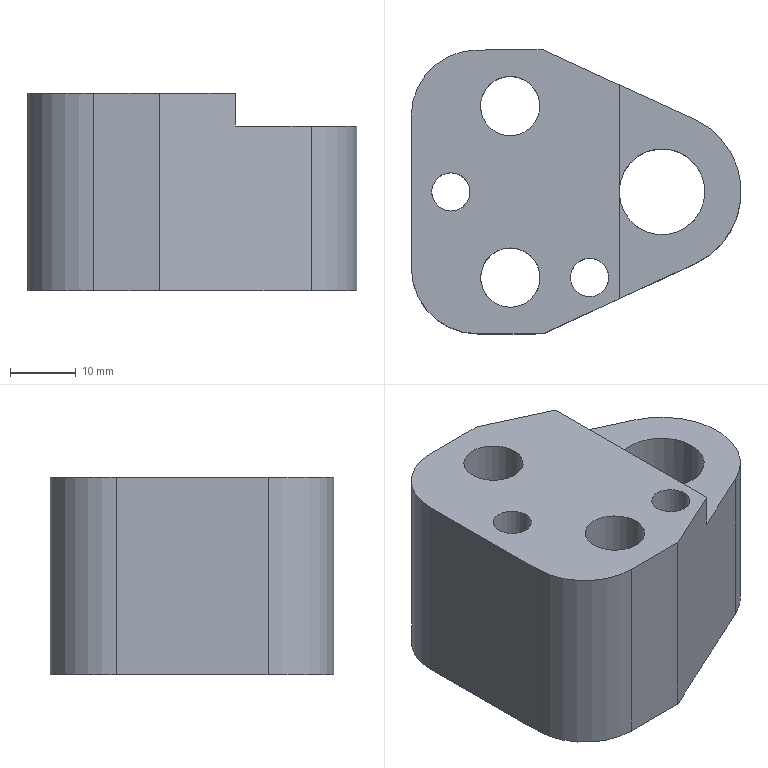Part | NX | features solid 2 | 1 solid | 27 faces | box 50.015 x 43.013 x 30 mm | volume 36579 mm3 | plane 15 | cylinder 12 | commonest cylinder face diameters 5.8 x2 8 x2 9 x2 14 x2 20 x2 13 x1
STEP:
#1=CARTESIAN_POINT('',(796.485,-52.747,102.));
#2=VERTEX_POINT('',#1);
#3=CARTESIAN_POINT('',(796.485,-52.747,127.));
#4=VERTEX_POINT('',#3);
#5=CARTESIAN_POINT('',(796.485,-52.747,102.));
#6=DIRECTION('',(0.,0.,1.));
#7=VECTOR('',#6,1000.);
#8=LINE('',#5,#7);
#9=EDGE_CURVE('',#2,#4,#8,.T.);
#10=ORIENTED_EDGE('',*,*,#9,.F.);
#11=CARTESIAN_POINT('',(796.485,-52.747,102.));
#12=VERTEX_POINT('',#11);
#13=CARTESIAN_POINT('',(796.471,-41.848,102.));
#14=DIRECTION('',(-0.001306,1.,0.));
#15=VECTOR('',#14,1000.);
#16=LINE('',#13,#15);
#17=EDGE_CURVE('',#2,#12,#16,.T.);
#18=ORIENTED_EDGE('',*,*,#17,.T.);
#19=CARTESIAN_POINT('',(796.485,-52.747,127.));
#20=VERTEX_POINT('',#19);
#21=CARTESIAN_POINT('',(796.485,-52.747,132.));
#22=DIRECTION('',(0.,0.,-1.));
#23=VECTOR('',#22,1000.);
#24=LINE('',#21,#23);
#25=EDGE_CURVE('',#20,#12,#24,.T.);
#26=ORIENTED_EDGE('',*,*,#25,.F.);
#27=CARTESIAN_POINT('',(796.471,-41.848,127.));
#28=DIRECTION('',(-0.001306,1.,0.));
#29=VECTOR('',#28,1000.);
#30=LINE('',#27,#29);
#31=EDGE_CURVE('',#4,#20,#30,.T.);
#32=ORIENTED_EDGE('',*,*,#31,.F.);
#33=EDGE_LOOP('',(#10,#18,#26,#32));
#34=FACE_BOUND('',#33,.T.);
#35=CARTESIAN_POINT('',(796.471,-41.848,102.));
#36=DIRECTION('',(1.,0.001306,0.));
#37=DIRECTION('',(0.,0.,1.));
#38=AXIS2_PLACEMENT_3D('',#35,#36,#37);
#39=PLANE('',#38);
#40=ADVANCED_FACE('',(#34),#39,.T.);
#41=CARTESIAN_POINT('',(773.479,-63.378,132.));
#42=VERTEX_POINT('',#41);
#43=CARTESIAN_POINT('',(784.972,-58.067,132.));
#44=VERTEX_POINT('',#43);
#45=CARTESIAN_POINT('',(791.635,-54.989,132.));
#46=DIRECTION('',(0.9078,0.4195,0.));
#47=VECTOR('',#46,1000.);
#48=LINE('',#45,#47);
#49=EDGE_CURVE('',#42,#44,#48,.T.);
#50=ORIENTED_EDGE('',*,*,#49,.T.);
#51=CARTESIAN_POINT('',(784.93,-25.659,132.));
#52=VERTEX_POINT('',#51);
#53=CARTESIAN_POINT('',(784.951,-41.863,132.));
#54=DIRECTION('',(-0.001306,1.,0.));
#55=VECTOR('',#54,1000.);
#56=LINE('',#53,#55);
#57=EDGE_CURVE('',#44,#52,#56,.T.);
#58=ORIENTED_EDGE('',*,*,#57,.T.);
#59=CARTESIAN_POINT('',(773.423,-20.378,132.));
#60=VERTEX_POINT('',#59);
#61=CARTESIAN_POINT('',(791.6,-28.72,132.));
#62=DIRECTION('',(-0.9089,0.4171,0.));
#63=VECTOR('',#62,1000.);
#64=LINE('',#61,#63);
#65=EDGE_CURVE('',#52,#60,#64,.T.);
#66=ORIENTED_EDGE('',*,*,#65,.T.);
#67=CARTESIAN_POINT('',(763.423,-20.391,132.));
#68=VERTEX_POINT('',#67);
#69=CARTESIAN_POINT('',(784.933,-20.363,132.));
#70=DIRECTION('',(1.,0.001306,0.));
#71=VECTOR('',#70,1000.);
#72=LINE('',#69,#71);
#73=EDGE_CURVE('',#68,#60,#72,.T.);
#74=ORIENTED_EDGE('',*,*,#73,.F.);
#75=CARTESIAN_POINT('',(753.436,-30.404,132.));
#76=VERTEX_POINT('',#75);
#77=CARTESIAN_POINT('',(763.436,-30.391,132.));
#78=DIRECTION('',(0.,0.,1.));
#79=DIRECTION('',(-1.,-0.002612,0.));
#80=AXIS2_PLACEMENT_3D('',#77,#78,#79);
#81=CIRCLE('',#80,10.);
#82=EDGE_CURVE('',#68,#76,#81,.T.);
#83=ORIENTED_EDGE('',*,*,#82,.T.);
#84=CARTESIAN_POINT('',(753.466,-53.404,132.));
#85=VERTEX_POINT('',#84);
#86=CARTESIAN_POINT('',(753.451,-41.904,132.));
#87=DIRECTION('',(-0.001306,1.,0.));
#88=VECTOR('',#87,1000.);
#89=LINE('',#86,#88);
#90=EDGE_CURVE('',#85,#76,#89,.T.);
#91=ORIENTED_EDGE('',*,*,#90,.F.);
#92=CARTESIAN_POINT('',(763.479,-63.391,132.));
#93=VERTEX_POINT('',#92);
#94=CARTESIAN_POINT('',(763.466,-53.391,132.));
#95=DIRECTION('',(0.,0.,1.));
#96=DIRECTION('',(-1.,-0.002612,0.));
#97=AXIS2_PLACEMENT_3D('',#94,#95,#96);
#98=CIRCLE('',#97,10.);
#99=EDGE_CURVE('',#85,#93,#98,.T.);
#100=ORIENTED_EDGE('',*,*,#99,.T.);
#101=CARTESIAN_POINT('',(784.989,-63.363,132.));
#102=DIRECTION('',(-1.,-0.001306,0.));
#103=VECTOR('',#102,1000.);
#104=LINE('',#101,#103);
#105=EDGE_CURVE('',#42,#93,#104,.T.);
#106=ORIENTED_EDGE('',*,*,#105,.F.);
#107=EDGE_LOOP('',(#50,#58,#66,#74,#83,#91,#100,#106));
#108=FACE_BOUND('',#107,.T.);
#109=CARTESIAN_POINT('',(759.447,-38.996,132.));
#110=VERTEX_POINT('',#109);
#111=CARTESIAN_POINT('',(759.451,-41.896,132.));
#112=DIRECTION('',(0.,0.,-1.));
#113=DIRECTION('',(-0.001306,1.,0.));
#114=AXIS2_PLACEMENT_3D('',#111,#112,#113);
#115=CIRCLE('',#114,2.9);
#116=EDGE_CURVE('',#110,#110,#115,.T.);
#117=ORIENTED_EDGE('',*,*,#116,.T.);
#118=EDGE_LOOP('',(#117));
#119=FACE_BOUND('',#118,.T.);
#120=CARTESIAN_POINT('',(780.464,-51.969,132.));
#121=VERTEX_POINT('',#120);
#122=CARTESIAN_POINT('',(780.468,-54.869,132.));
#123=DIRECTION('',(0.,0.,-1.));
#124=DIRECTION('',(-0.001306,1.,0.));
#125=AXIS2_PLACEMENT_3D('',#122,#123,#124);
#126=CIRCLE('',#125,2.9);
#127=EDGE_CURVE('',#121,#121,#126,.T.);
#128=ORIENTED_EDGE('',*,*,#127,.T.);
#129=EDGE_LOOP('',(#128));
#130=FACE_BOUND('',#129,.T.);
#131=CARTESIAN_POINT('',(768.462,-50.384,132.));
#132=VERTEX_POINT('',#131);
#133=CARTESIAN_POINT('',(768.468,-54.884,132.));
#134=DIRECTION('',(0.,0.,-1.));
#135=DIRECTION('',(-0.001306,1.,0.));
#136=AXIS2_PLACEMENT_3D('',#133,#134,#135);
#137=CIRCLE('',#136,4.5);
#138=EDGE_CURVE('',#132,#132,#137,.T.);
#139=ORIENTED_EDGE('',*,*,#138,.T.);
#140=EDGE_LOOP('',(#139));
#141=FACE_BOUND('',#140,.T.);
#142=CARTESIAN_POINT('',(768.428,-24.384,132.));
#143=VERTEX_POINT('',#142);
#144=CARTESIAN_POINT('',(768.434,-28.884,132.));
#145=DIRECTION('',(0.,0.,-1.));
#146=DIRECTION('',(-0.001306,1.,0.));
#147=AXIS2_PLACEMENT_3D('',#144,#145,#146);
#148=CIRCLE('',#147,4.5);
#149=EDGE_CURVE('',#143,#143,#148,.T.);
#150=ORIENTED_EDGE('',*,*,#149,.T.);
#151=EDGE_LOOP('',(#150));
#152=FACE_BOUND('',#151,.T.);
#153=CARTESIAN_POINT('',(784.961,-41.863,132.));
#154=DIRECTION('',(0.,0.,1.));
#155=DIRECTION('',(0.001306,-1.,0.));
#156=AXIS2_PLACEMENT_3D('',#153,#154,#155);
#157=PLANE('',#156);
#158=ADVANCED_FACE('',(#108,#119,#130,#141,#152),#157,.T.);
#159=CARTESIAN_POINT('',(773.423,-20.378,102.));
#160=VERTEX_POINT('',#159);
#161=CARTESIAN_POINT('',(773.423,-20.378,102.));
#162=DIRECTION('',(0.,0.,1.));
#163=VECTOR('',#162,1000.);
#164=LINE('',#161,#163);
#165=EDGE_CURVE('',#160,#60,#164,.T.);
#166=ORIENTED_EDGE('',*,*,#165,.F.);
#167=CARTESIAN_POINT('',(763.423,-20.391,102.));
#168=VERTEX_POINT('',#167);
#169=CARTESIAN_POINT('',(784.933,-20.363,102.));
#170=DIRECTION('',(-1.,-0.001306,0.));
#171=VECTOR('',#170,1000.);
#172=LINE('',#169,#171);
#173=EDGE_CURVE('',#160,#168,#172,.T.);
#174=ORIENTED_EDGE('',*,*,#173,.T.);
#175=CARTESIAN_POINT('',(763.423,-20.391,102.));
#176=DIRECTION('',(0.,0.,1.));
#177=VECTOR('',#176,1000.);
#178=LINE('',#175,#177);
#179=EDGE_CURVE('',#168,#68,#178,.T.);
#180=ORIENTED_EDGE('',*,*,#179,.T.);
#181=ORIENTED_EDGE('',*,*,#73,.T.);
#182=EDGE_LOOP('',(#166,#174,#180,#181));
#183=FACE_BOUND('',#182,.T.);
#184=CARTESIAN_POINT('',(784.933,-20.363,102.));
#185=DIRECTION('',(-0.001306,1.,0.));
#186=DIRECTION('',(0.,0.,1.));
#187=AXIS2_PLACEMENT_3D('',#184,#185,#186);
#188=PLANE('',#187);
#189=ADVANCED_FACE('',(#183),#188,.T.);
#190=CARTESIAN_POINT('',(796.457,-30.948,127.));
#191=VERTEX_POINT('',#190);
#192=CARTESIAN_POINT('',(796.457,-30.948,102.));
#193=VERTEX_POINT('',#192);
#194=CARTESIAN_POINT('',(796.457,-30.948,102.));
#195=DIRECTION('',(0.,0.,-1.));
#196=VECTOR('',#195,1000.);
#197=LINE('',#194,#196);
#198=EDGE_CURVE('',#191,#193,#197,.T.);
#199=ORIENTED_EDGE('',*,*,#198,.F.);
#200=CARTESIAN_POINT('',(796.457,-30.948,127.));
#201=VERTEX_POINT('',#200);
#202=CARTESIAN_POINT('',(796.471,-41.848,127.));
#203=DIRECTION('',(-0.001306,1.,0.));
#204=VECTOR('',#203,1000.);
#205=LINE('',#202,#204);
#206=EDGE_CURVE('',#201,#191,#205,.T.);
#207=ORIENTED_EDGE('',*,*,#206,.F.);
#208=CARTESIAN_POINT('',(796.457,-30.948,102.));
#209=VERTEX_POINT('',#208);
#210=CARTESIAN_POINT('',(796.457,-30.948,132.));
#211=DIRECTION('',(0.,0.,-1.));
#212=VECTOR('',#211,1000.);
#213=LINE('',#210,#212);
#214=EDGE_CURVE('',#209,#201,#213,.F.);
#215=ORIENTED_EDGE('',*,*,#214,.F.);
#216=CARTESIAN_POINT('',(796.471,-41.848,102.));
#217=DIRECTION('',(-0.001306,1.,0.));
#218=VECTOR('',#217,1000.);
#219=LINE('',#216,#218);
#220=EDGE_CURVE('',#209,#193,#219,.T.);
#221=ORIENTED_EDGE('',*,*,#220,.T.);
#222=EDGE_LOOP('',(#199,#207,#215,#221));
#223=FACE_BOUND('',#222,.T.);
#224=CARTESIAN_POINT('',(796.471,-41.848,102.));
#225=DIRECTION('',(1.,0.001306,0.));
#226=DIRECTION('',(0.,0.,1.));
#227=AXIS2_PLACEMENT_3D('',#224,#225,#226);
#228=PLANE('',#227);
#229=ADVANCED_FACE('',(#223),#228,.T.);
#230=CARTESIAN_POINT('',(773.479,-63.378,102.));
#231=VERTEX_POINT('',#230);
#232=CARTESIAN_POINT('',(791.635,-54.989,102.));
#233=DIRECTION('',(-0.9078,-0.4195,0.));
#234=VECTOR('',#233,1000.);
#235=LINE('',#232,#234);
#236=EDGE_CURVE('',#2,#231,#235,.T.);
#237=ORIENTED_EDGE('',*,*,#236,.T.);
#238=CARTESIAN_POINT('',(763.479,-63.391,102.));
#239=VERTEX_POINT('',#238);
#240=CARTESIAN_POINT('',(784.989,-63.363,102.));
#241=DIRECTION('',(1.,0.001306,0.));
#242=VECTOR('',#241,1000.);
#243=LINE('',#240,#242);
#244=EDGE_CURVE('',#239,#231,#243,.T.);
#245=ORIENTED_EDGE('',*,*,#244,.F.);
#246=CARTESIAN_POINT('',(753.466,-53.404,102.));
#247=VERTEX_POINT('',#246);
#248=CARTESIAN_POINT('',(763.466,-53.391,102.));
#249=DIRECTION('',(0.,0.,-1.));
#250=DIRECTION('',(1.,0.002612,0.));
#251=AXIS2_PLACEMENT_3D('',#248,#249,#250);
#252=CIRCLE('',#251,10.);
#253=EDGE_CURVE('',#239,#247,#252,.T.);
#254=ORIENTED_EDGE('',*,*,#253,.T.);
#255=CARTESIAN_POINT('',(753.436,-30.404,102.));
#256=VERTEX_POINT('',#255);
#257=CARTESIAN_POINT('',(753.451,-41.904,102.));
#258=DIRECTION('',(0.001306,-1.,0.));
#259=VECTOR('',#258,1000.);
#260=LINE('',#257,#259);
#261=EDGE_CURVE('',#256,#247,#260,.T.);
#262=ORIENTED_EDGE('',*,*,#261,.F.);
#263=CARTESIAN_POINT('',(763.436,-30.391,102.));
#264=DIRECTION('',(0.,0.,-1.));
#265=DIRECTION('',(1.,0.002612,0.));
#266=AXIS2_PLACEMENT_3D('',#263,#264,#265);
#267=CIRCLE('',#266,10.);
#268=EDGE_CURVE('',#256,#168,#267,.T.);
#269=ORIENTED_EDGE('',*,*,#268,.T.);
#270=ORIENTED_EDGE('',*,*,#173,.F.);
#271=CARTESIAN_POINT('',(791.6,-28.72,102.));
#272=DIRECTION('',(0.9089,-0.4171,0.));
#273=VECTOR('',#272,1000.);
#274=LINE('',#271,#273);
#275=EDGE_CURVE('',#160,#193,#274,.T.);
#276=ORIENTED_EDGE('',*,*,#275,.T.);
#277=ORIENTED_EDGE('',*,*,#220,.F.);
#278=CARTESIAN_POINT('',(791.451,-41.854,102.));
#279=DIRECTION('',(0.,0.,1.));
#280=DIRECTION('',(0.001306,-1.,0.));
#281=AXIS2_PLACEMENT_3D('',#278,#279,#280);
#282=CIRCLE('',#281,12.);
#283=EDGE_CURVE('',#12,#209,#282,.T.);
#284=ORIENTED_EDGE('',*,*,#283,.F.);
#285=ORIENTED_EDGE('',*,*,#17,.F.);
#286=EDGE_LOOP('',(#237,#245,#254,#262,#269,#270,#276,#277,#284,#285));
#287=FACE_BOUND('',#286,.T.);
#288=CARTESIAN_POINT('',(759.456,-45.896,102.));
#289=VERTEX_POINT('',#288);
#290=CARTESIAN_POINT('',(759.451,-41.896,102.));
#291=DIRECTION('',(0.,0.,1.));
#292=DIRECTION('',(0.001306,-1.,0.));
#293=AXIS2_PLACEMENT_3D('',#290,#291,#292);
#294=CIRCLE('',#293,4.);
#295=EDGE_CURVE('',#289,#289,#294,.T.);
#296=ORIENTED_EDGE('',*,*,#295,.T.);
#297=EDGE_LOOP('',(#296));
#298=FACE_BOUND('',#297,.T.);
#299=CARTESIAN_POINT('',(780.473,-58.869,102.));
#300=VERTEX_POINT('',#299);
#301=CARTESIAN_POINT('',(780.468,-54.869,102.));
#302=DIRECTION('',(0.,0.,1.));
#303=DIRECTION('',(0.001306,-1.,0.));
#304=AXIS2_PLACEMENT_3D('',#301,#302,#303);
#305=CIRCLE('',#304,4.);
#306=EDGE_CURVE('',#300,#300,#305,.T.);
#307=ORIENTED_EDGE('',*,*,#306,.T.);
#308=EDGE_LOOP('',(#307));
#309=FACE_BOUND('',#308,.T.);
#310=CARTESIAN_POINT('',(768.477,-61.884,102.));
#311=VERTEX_POINT('',#310);
#312=CARTESIAN_POINT('',(768.468,-54.884,102.));
#313=DIRECTION('',(0.,0.,1.));
#314=DIRECTION('',(0.001306,-1.,0.));
#315=AXIS2_PLACEMENT_3D('',#312,#313,#314);
#316=CIRCLE('',#315,7.);
#317=EDGE_CURVE('',#311,#311,#316,.T.);
#318=ORIENTED_EDGE('',*,*,#317,.T.);
#319=EDGE_LOOP('',(#318));
#320=FACE_BOUND('',#319,.T.);
#321=CARTESIAN_POINT('',(768.443,-35.884,102.));
#322=VERTEX_POINT('',#321);
#323=CARTESIAN_POINT('',(768.434,-28.884,102.));
#324=DIRECTION('',(0.,0.,1.));
#325=DIRECTION('',(0.001306,-1.,0.));
#326=AXIS2_PLACEMENT_3D('',#323,#324,#325);
#327=CIRCLE('',#326,7.);
#328=EDGE_CURVE('',#322,#322,#327,.T.);
#329=ORIENTED_EDGE('',*,*,#328,.T.);
#330=EDGE_LOOP('',(#329));
#331=FACE_BOUND('',#330,.T.);
#332=CARTESIAN_POINT('',(791.46,-48.354,102.));
#333=VERTEX_POINT('',#332);
#334=CARTESIAN_POINT('',(791.451,-41.854,102.));
#335=DIRECTION('',(0.,0.,1.));
#336=DIRECTION('',(0.001306,-1.,0.));
#337=AXIS2_PLACEMENT_3D('',#334,#335,#336);
#338=CIRCLE('',#337,6.5);
#339=EDGE_CURVE('',#333,#333,#338,.T.);
#340=ORIENTED_EDGE('',*,*,#339,.T.);
#341=EDGE_LOOP('',(#340));
#342=FACE_BOUND('',#341,.T.);
#343=CARTESIAN_POINT('',(784.961,-41.863,102.));
#344=DIRECTION('',(0.,0.,-1.));
#345=DIRECTION('',(-0.001306,1.,0.));
#346=AXIS2_PLACEMENT_3D('',#343,#344,#345);
#347=PLANE('',#346);
#348=ADVANCED_FACE('',(#287,#298,#309,#320,#331,#342),#347,.T.);
#349=CARTESIAN_POINT('',(773.479,-63.378,102.));
#350=DIRECTION('',(0.,0.,1.));
#351=VECTOR('',#350,1000.);
#352=LINE('',#349,#351);
#353=EDGE_CURVE('',#231,#42,#352,.T.);
#354=ORIENTED_EDGE('',*,*,#353,.T.);
#355=ORIENTED_EDGE('',*,*,#105,.T.);
#356=CARTESIAN_POINT('',(763.479,-63.391,102.));
#357=DIRECTION('',(0.,0.,1.));
#358=VECTOR('',#357,1000.);
#359=LINE('',#356,#358);
#360=EDGE_CURVE('',#93,#239,#359,.F.);
#361=ORIENTED_EDGE('',*,*,#360,.T.);
#362=ORIENTED_EDGE('',*,*,#244,.T.);
#363=EDGE_LOOP('',(#354,#355,#361,#362));
#364=FACE_BOUND('',#363,.T.);
#365=CARTESIAN_POINT('',(784.989,-63.363,102.));
#366=DIRECTION('',(0.001306,-1.,0.));
#367=DIRECTION('',(0.,0.,-1.));
#368=AXIS2_PLACEMENT_3D('',#365,#366,#367);
#369=PLANE('',#368);
#370=ADVANCED_FACE('',(#364),#369,.T.);
#371=CARTESIAN_POINT('',(791.451,-41.854,127.));
#372=DIRECTION('',(0.,0.,-1.));
#373=DIRECTION('',(1.,0.002612,0.));
#374=AXIS2_PLACEMENT_3D('',#371,#372,#373);
#375=CIRCLE('',#374,12.);
#376=EDGE_CURVE('',#20,#201,#375,.F.);
#377=ORIENTED_EDGE('',*,*,#376,.F.);
#378=ORIENTED_EDGE('',*,*,#25,.T.);
#379=ORIENTED_EDGE('',*,*,#283,.T.);
#380=ORIENTED_EDGE('',*,*,#214,.T.);
#381=EDGE_LOOP('',(#377,#378,#379,#380));
#382=FACE_BOUND('',#381,.T.);
#383=CARTESIAN_POINT('',(791.451,-41.854,132.));
#384=DIRECTION('',(0.,0.,-1.));
#385=DIRECTION('',(-0.001306,1.,0.));
#386=AXIS2_PLACEMENT_3D('',#383,#384,#385);
#387=CYLINDRICAL_SURFACE('',#386,12.);
#388=ADVANCED_FACE('',(#382),#387,.T.);
#389=ORIENTED_EDGE('',*,*,#261,.T.);
#390=CARTESIAN_POINT('',(753.466,-53.404,102.));
#391=DIRECTION('',(0.,0.,1.));
#392=VECTOR('',#391,1000.);
#393=LINE('',#390,#392);
#394=EDGE_CURVE('',#247,#85,#393,.T.);
#395=ORIENTED_EDGE('',*,*,#394,.T.);
#396=ORIENTED_EDGE('',*,*,#90,.T.);
#397=CARTESIAN_POINT('',(753.436,-30.404,102.));
#398=DIRECTION('',(0.,0.,1.));
#399=VECTOR('',#398,1000.);
#400=LINE('',#397,#399);
#401=EDGE_CURVE('',#76,#256,#400,.F.);
#402=ORIENTED_EDGE('',*,*,#401,.T.);
#403=EDGE_LOOP('',(#389,#395,#396,#402));
#404=FACE_BOUND('',#403,.T.);
#405=CARTESIAN_POINT('',(753.451,-41.904,102.));
#406=DIRECTION('',(-1.,-0.001306,0.));
#407=DIRECTION('',(0.,0.,-1.));
#408=AXIS2_PLACEMENT_3D('',#405,#406,#407);
#409=PLANE('',#408);
#410=ADVANCED_FACE('',(#404),#409,.T.);
#411=ORIENTED_EDGE('',*,*,#57,.F.);
#412=CARTESIAN_POINT('',(784.972,-58.067,127.));
#413=VERTEX_POINT('',#412);
#414=CARTESIAN_POINT('',(784.972,-58.067,127.));
#415=DIRECTION('',(0.,0.,-1.));
#416=VECTOR('',#415,1000.);
#417=LINE('',#414,#416);
#418=EDGE_CURVE('',#44,#413,#417,.T.);
#419=ORIENTED_EDGE('',*,*,#418,.T.);
#420=CARTESIAN_POINT('',(784.951,-41.863,127.));
#421=VERTEX_POINT('',#420);
#422=CARTESIAN_POINT('',(784.951,-41.863,127.));
#423=DIRECTION('',(0.001306,-1.,0.));
#424=VECTOR('',#423,1000.);
#425=LINE('',#422,#424);
#426=EDGE_CURVE('',#421,#413,#425,.T.);
#427=ORIENTED_EDGE('',*,*,#426,.F.);
#428=CARTESIAN_POINT('',(784.93,-25.659,127.));
#429=VERTEX_POINT('',#428);
#430=CARTESIAN_POINT('',(784.951,-41.863,127.));
#431=DIRECTION('',(0.001306,-1.,0.));
#432=VECTOR('',#431,1000.);
#433=LINE('',#430,#432);
#434=EDGE_CURVE('',#429,#421,#433,.T.);
#435=ORIENTED_EDGE('',*,*,#434,.F.);
#436=CARTESIAN_POINT('',(784.93,-25.659,127.));
#437=DIRECTION('',(0.,0.,1.));
#438=VECTOR('',#437,1000.);
#439=LINE('',#436,#438);
#440=EDGE_CURVE('',#429,#52,#439,.T.);
#441=ORIENTED_EDGE('',*,*,#440,.T.);
#442=EDGE_LOOP('',(#411,#419,#427,#435,#441));
#443=FACE_BOUND('',#442,.T.);
#444=CARTESIAN_POINT('',(784.951,-41.863,127.));
#445=DIRECTION('',(-1.,-0.001306,0.));
#446=DIRECTION('',(0.,0.,-1.));
#447=AXIS2_PLACEMENT_3D('',#444,#445,#446);
#448=PLANE('',#447);
#449=ADVANCED_FACE('',(#443),#448,.F.);
#450=ORIENTED_EDGE('',*,*,#426,.T.);
#451=CARTESIAN_POINT('',(813.8,-44.747,127.));
#452=DIRECTION('',(0.9078,0.4195,0.));
#453=VECTOR('',#452,1000.);
#454=LINE('',#451,#453);
#455=EDGE_CURVE('',#413,#4,#454,.T.);
#456=ORIENTED_EDGE('',*,*,#455,.T.);
#457=ORIENTED_EDGE('',*,*,#31,.T.);
#458=ORIENTED_EDGE('',*,*,#376,.T.);
#459=ORIENTED_EDGE('',*,*,#206,.T.);
#460=CARTESIAN_POINT('',(813.793,-38.904,127.));
#461=DIRECTION('',(-0.9089,0.4171,0.));
#462=VECTOR('',#461,1000.);
#463=LINE('',#460,#462);
#464=EDGE_CURVE('',#191,#429,#463,.T.);
#465=ORIENTED_EDGE('',*,*,#464,.T.);
#466=ORIENTED_EDGE('',*,*,#434,.T.);
#467=CARTESIAN_POINT('',(791.451,-41.854,127.));
#468=DIRECTION('',(0.,0.,-1.));
#469=DIRECTION('',(-0.001306,1.,0.));
#470=AXIS2_PLACEMENT_3D('',#467,#468,#469);
#471=CIRCLE('',#470,6.5);
#472=EDGE_CURVE('',#421,#421,#471,.T.);
#473=ORIENTED_EDGE('',*,*,#472,.T.);
#474=EDGE_LOOP('',(#450,#456,#457,#458,#459,#465,#466,#473));
#475=FACE_BOUND('',#474,.T.);
#476=CARTESIAN_POINT('',(812.451,-41.827,127.));
#477=DIRECTION('',(0.,0.,-1.));
#478=DIRECTION('',(-0.001306,1.,0.));
#479=AXIS2_PLACEMENT_3D('',#476,#477,#478);
#480=PLANE('',#479);
#481=ADVANCED_FACE('',(#475),#480,.F.);
#482=ORIENTED_EDGE('',*,*,#339,.F.);
#483=EDGE_LOOP('',(#482));
#484=FACE_BOUND('',#483,.T.);
#485=ORIENTED_EDGE('',*,*,#472,.F.);
#486=EDGE_LOOP('',(#485));
#487=FACE_BOUND('',#486,.T.);
#488=CARTESIAN_POINT('',(791.451,-41.854,127.));
#489=DIRECTION('',(0.,0.,-1.));
#490=DIRECTION('',(-0.001306,1.,0.));
#491=AXIS2_PLACEMENT_3D('',#488,#489,#490);
#492=CYLINDRICAL_SURFACE('',#491,6.5);
#493=ADVANCED_FACE('',(#484,#487),#492,.F.);
#494=CARTESIAN_POINT('',(763.934,-28.896,112.));
#495=VERTEX_POINT('',#494);
#496=CARTESIAN_POINT('',(768.434,-28.884,112.));
#497=DIRECTION('',(0.,0.,1.));
#498=DIRECTION('',(-1.,-0.002612,0.));
#499=AXIS2_PLACEMENT_3D('',#496,#497,#498);
#500=CIRCLE('',#499,4.5);
#501=EDGE_CURVE('',#495,#495,#500,.F.);
#502=ORIENTED_EDGE('',*,*,#501,.T.);
#503=EDGE_LOOP('',(#502));
#504=FACE_BOUND('',#503,.T.);
#505=ORIENTED_EDGE('',*,*,#149,.F.);
#506=EDGE_LOOP('',(#505));
#507=FACE_BOUND('',#506,.T.);
#508=CARTESIAN_POINT('',(768.434,-28.884,132.));
#509=DIRECTION('',(0.,0.,-1.));
#510=DIRECTION('',(-0.001306,1.,0.));
#511=AXIS2_PLACEMENT_3D('',#508,#509,#510);
#512=CYLINDRICAL_SURFACE('',#511,4.5);
#513=ADVANCED_FACE('',(#504,#507),#512,.F.);
#514=CARTESIAN_POINT('',(768.425,-21.884,112.));
#515=VERTEX_POINT('',#514);
#516=CARTESIAN_POINT('',(768.434,-28.884,112.));
#517=DIRECTION('',(0.,0.,-1.));
#518=DIRECTION('',(-0.001306,1.,0.));
#519=AXIS2_PLACEMENT_3D('',#516,#517,#518);
#520=CIRCLE('',#519,7.);
#521=EDGE_CURVE('',#515,#515,#520,.T.);
#522=ORIENTED_EDGE('',*,*,#521,.T.);
#523=EDGE_LOOP('',(#522));
#524=FACE_BOUND('',#523,.T.);
#525=ORIENTED_EDGE('',*,*,#501,.F.);
#526=EDGE_LOOP('',(#525));
#527=FACE_BOUND('',#526,.T.);
#528=CARTESIAN_POINT('',(768.434,-28.884,112.));
#529=DIRECTION('',(0.,0.,1.));
#530=DIRECTION('',(0.001306,-1.,0.));
#531=AXIS2_PLACEMENT_3D('',#528,#529,#530);
#532=PLANE('',#531);
#533=ADVANCED_FACE('',(#524,#527),#532,.F.);
#534=ORIENTED_EDGE('',*,*,#328,.F.);
#535=EDGE_LOOP('',(#534));
#536=FACE_BOUND('',#535,.T.);
#537=ORIENTED_EDGE('',*,*,#521,.F.);
#538=EDGE_LOOP('',(#537));
#539=FACE_BOUND('',#538,.T.);
#540=CARTESIAN_POINT('',(768.434,-28.884,112.));
#541=DIRECTION('',(0.,0.,-1.));
#542=DIRECTION('',(-0.001306,1.,0.));
#543=AXIS2_PLACEMENT_3D('',#540,#541,#542);
#544=CYLINDRICAL_SURFACE('',#543,7.);
#545=ADVANCED_FACE('',(#536,#539),#544,.F.);
#546=CARTESIAN_POINT('',(763.968,-54.896,112.));
#547=VERTEX_POINT('',#546);
#548=CARTESIAN_POINT('',(768.468,-54.884,112.));
#549=DIRECTION('',(0.,0.,1.));
#550=DIRECTION('',(-1.,-0.002612,0.));
#551=AXIS2_PLACEMENT_3D('',#548,#549,#550);
#552=CIRCLE('',#551,4.5);
#553=EDGE_CURVE('',#547,#547,#552,.F.);
#554=ORIENTED_EDGE('',*,*,#553,.T.);
#555=EDGE_LOOP('',(#554));
#556=FACE_BOUND('',#555,.T.);
#557=ORIENTED_EDGE('',*,*,#138,.F.);
#558=EDGE_LOOP('',(#557));
#559=FACE_BOUND('',#558,.T.);
#560=CARTESIAN_POINT('',(768.468,-54.884,132.));
#561=DIRECTION('',(0.,0.,-1.));
#562=DIRECTION('',(-0.001306,1.,0.));
#563=AXIS2_PLACEMENT_3D('',#560,#561,#562);
#564=CYLINDRICAL_SURFACE('',#563,4.5);
#565=ADVANCED_FACE('',(#556,#559),#564,.F.);
#566=CARTESIAN_POINT('',(768.459,-47.884,112.));
#567=VERTEX_POINT('',#566);
#568=CARTESIAN_POINT('',(768.468,-54.884,112.));
#569=DIRECTION('',(0.,0.,-1.));
#570=DIRECTION('',(-0.001306,1.,0.));
#571=AXIS2_PLACEMENT_3D('',#568,#569,#570);
#572=CIRCLE('',#571,7.);
#573=EDGE_CURVE('',#567,#567,#572,.T.);
#574=ORIENTED_EDGE('',*,*,#573,.T.);
#575=EDGE_LOOP('',(#574));
#576=FACE_BOUND('',#575,.T.);
#577=ORIENTED_EDGE('',*,*,#553,.F.);
#578=EDGE_LOOP('',(#577));
#579=FACE_BOUND('',#578,.T.);
#580=CARTESIAN_POINT('',(768.468,-54.884,112.));
#581=DIRECTION('',(0.,0.,1.));
#582=DIRECTION('',(0.001306,-1.,0.));
#583=AXIS2_PLACEMENT_3D('',#580,#581,#582);
#584=PLANE('',#583);
#585=ADVANCED_FACE('',(#576,#579),#584,.F.);
#586=ORIENTED_EDGE('',*,*,#317,.F.);
#587=EDGE_LOOP('',(#586));
#588=FACE_BOUND('',#587,.T.);
#589=ORIENTED_EDGE('',*,*,#573,.F.);
#590=EDGE_LOOP('',(#589));
#591=FACE_BOUND('',#590,.T.);
#592=CARTESIAN_POINT('',(768.468,-54.884,112.));
#593=DIRECTION('',(0.,0.,-1.));
#594=DIRECTION('',(-0.001306,1.,0.));
#595=AXIS2_PLACEMENT_3D('',#592,#593,#594);
#596=CYLINDRICAL_SURFACE('',#595,7.);
#597=ADVANCED_FACE('',(#588,#591),#596,.F.);
#598=CARTESIAN_POINT('',(777.568,-54.876,122.));
#599=VERTEX_POINT('',#598);
#600=CARTESIAN_POINT('',(780.468,-54.869,122.));
#601=DIRECTION('',(0.,0.,1.));
#602=DIRECTION('',(-1.,-0.002612,0.));
#603=AXIS2_PLACEMENT_3D('',#600,#601,#602);
#604=CIRCLE('',#603,2.9);
#605=EDGE_CURVE('',#599,#599,#604,.F.);
#606=ORIENTED_EDGE('',*,*,#605,.T.);
#607=EDGE_LOOP('',(#606));
#608=FACE_BOUND('',#607,.T.);
#609=ORIENTED_EDGE('',*,*,#127,.F.);
#610=EDGE_LOOP('',(#609));
#611=FACE_BOUND('',#610,.T.);
#612=CARTESIAN_POINT('',(780.468,-54.869,132.));
#613=DIRECTION('',(0.,0.,-1.));
#614=DIRECTION('',(-0.001306,1.,0.));
#615=AXIS2_PLACEMENT_3D('',#612,#613,#614);
#616=CYLINDRICAL_SURFACE('',#615,2.9);
#617=ADVANCED_FACE('',(#608,#611),#616,.F.);
#618=CARTESIAN_POINT('',(780.463,-50.869,122.));
#619=VERTEX_POINT('',#618);
#620=CARTESIAN_POINT('',(780.468,-54.869,122.));
#621=DIRECTION('',(0.,0.,-1.));
#622=DIRECTION('',(-0.001306,1.,0.));
#623=AXIS2_PLACEMENT_3D('',#620,#621,#622);
#624=CIRCLE('',#623,4.);
#625=EDGE_CURVE('',#619,#619,#624,.T.);
#626=ORIENTED_EDGE('',*,*,#625,.T.);
#627=EDGE_LOOP('',(#626));
#628=FACE_BOUND('',#627,.T.);
#629=ORIENTED_EDGE('',*,*,#605,.F.);
#630=EDGE_LOOP('',(#629));
#631=FACE_BOUND('',#630,.T.);
#632=CARTESIAN_POINT('',(780.468,-54.869,122.));
#633=DIRECTION('',(0.,0.,1.));
#634=DIRECTION('',(0.001306,-1.,0.));
#635=AXIS2_PLACEMENT_3D('',#632,#633,#634);
#636=PLANE('',#635);
#637=ADVANCED_FACE('',(#628,#631),#636,.F.);
#638=ORIENTED_EDGE('',*,*,#306,.F.);
#639=EDGE_LOOP('',(#638));
#640=FACE_BOUND('',#639,.T.);
#641=ORIENTED_EDGE('',*,*,#625,.F.);
#642=EDGE_LOOP('',(#641));
#643=FACE_BOUND('',#642,.T.);
#644=CARTESIAN_POINT('',(780.468,-54.869,122.));
#645=DIRECTION('',(0.,0.,-1.));
#646=DIRECTION('',(-0.001306,1.,0.));
#647=AXIS2_PLACEMENT_3D('',#644,#645,#646);
#648=CYLINDRICAL_SURFACE('',#647,4.);
#649=ADVANCED_FACE('',(#640,#643),#648,.F.);
#650=CARTESIAN_POINT('',(756.551,-41.904,122.));
#651=VERTEX_POINT('',#650);
#652=CARTESIAN_POINT('',(759.451,-41.896,122.));
#653=DIRECTION('',(0.,0.,1.));
#654=DIRECTION('',(-1.,-0.002612,0.));
#655=AXIS2_PLACEMENT_3D('',#652,#653,#654);
#656=CIRCLE('',#655,2.9);
#657=EDGE_CURVE('',#651,#651,#656,.F.);
#658=ORIENTED_EDGE('',*,*,#657,.T.);
#659=EDGE_LOOP('',(#658));
#660=FACE_BOUND('',#659,.T.);
#661=ORIENTED_EDGE('',*,*,#116,.F.);
#662=EDGE_LOOP('',(#661));
#663=FACE_BOUND('',#662,.T.);
#664=CARTESIAN_POINT('',(759.451,-41.896,132.));
#665=DIRECTION('',(0.,0.,-1.));
#666=DIRECTION('',(-0.001306,1.,0.));
#667=AXIS2_PLACEMENT_3D('',#664,#665,#666);
#668=CYLINDRICAL_SURFACE('',#667,2.9);
#669=ADVANCED_FACE('',(#660,#663),#668,.F.);
#670=CARTESIAN_POINT('',(759.446,-37.896,122.));
#671=VERTEX_POINT('',#670);
#672=CARTESIAN_POINT('',(759.451,-41.896,122.));
#673=DIRECTION('',(0.,0.,-1.));
#674=DIRECTION('',(-0.001306,1.,0.));
#675=AXIS2_PLACEMENT_3D('',#672,#673,#674);
#676=CIRCLE('',#675,4.);
#677=EDGE_CURVE('',#671,#671,#676,.T.);
#678=ORIENTED_EDGE('',*,*,#677,.T.);
#679=EDGE_LOOP('',(#678));
#680=FACE_BOUND('',#679,.T.);
#681=ORIENTED_EDGE('',*,*,#657,.F.);
#682=EDGE_LOOP('',(#681));
#683=FACE_BOUND('',#682,.T.);
#684=CARTESIAN_POINT('',(759.451,-41.896,122.));
#685=DIRECTION('',(0.,0.,1.));
#686=DIRECTION('',(0.001306,-1.,0.));
#687=AXIS2_PLACEMENT_3D('',#684,#685,#686);
#688=PLANE('',#687);
#689=ADVANCED_FACE('',(#680,#683),#688,.F.);
#690=ORIENTED_EDGE('',*,*,#295,.F.);
#691=EDGE_LOOP('',(#690));
#692=FACE_BOUND('',#691,.T.);
#693=ORIENTED_EDGE('',*,*,#677,.F.);
#694=EDGE_LOOP('',(#693));
#695=FACE_BOUND('',#694,.T.);
#696=CARTESIAN_POINT('',(759.451,-41.896,122.));
#697=DIRECTION('',(0.,0.,-1.));
#698=DIRECTION('',(-0.001306,1.,0.));
#699=AXIS2_PLACEMENT_3D('',#696,#697,#698);
#700=CYLINDRICAL_SURFACE('',#699,4.);
#701=ADVANCED_FACE('',(#692,#695),#700,.F.);
#702=ORIENTED_EDGE('',*,*,#253,.F.);
#703=ORIENTED_EDGE('',*,*,#360,.F.);
#704=ORIENTED_EDGE('',*,*,#99,.F.);
#705=ORIENTED_EDGE('',*,*,#394,.F.);
#706=EDGE_LOOP('',(#702,#703,#704,#705));
#707=FACE_BOUND('',#706,.T.);
#708=CARTESIAN_POINT('',(763.466,-53.391,102.));
#709=DIRECTION('',(0.,0.,1.));
#710=DIRECTION('',(-1.,-0.002612,0.));
#711=AXIS2_PLACEMENT_3D('',#708,#709,#710);
#712=CYLINDRICAL_SURFACE('',#711,10.);
#713=ADVANCED_FACE('',(#707),#712,.T.);
#714=ORIENTED_EDGE('',*,*,#268,.F.);
#715=ORIENTED_EDGE('',*,*,#401,.F.);
#716=ORIENTED_EDGE('',*,*,#82,.F.);
#717=ORIENTED_EDGE('',*,*,#179,.F.);
#718=EDGE_LOOP('',(#714,#715,#716,#717));
#719=FACE_BOUND('',#718,.T.);
#720=CARTESIAN_POINT('',(763.436,-30.391,102.));
#721=DIRECTION('',(0.,0.,1.));
#722=DIRECTION('',(-1.,-0.002612,0.));
#723=AXIS2_PLACEMENT_3D('',#720,#721,#722);
#724=CYLINDRICAL_SURFACE('',#723,10.);
#725=ADVANCED_FACE('',(#719),#724,.T.);
#726=ORIENTED_EDGE('',*,*,#198,.T.);
#727=ORIENTED_EDGE('',*,*,#275,.F.);
#728=ORIENTED_EDGE('',*,*,#165,.T.);
#729=ORIENTED_EDGE('',*,*,#65,.F.);
#730=ORIENTED_EDGE('',*,*,#440,.F.);
#731=ORIENTED_EDGE('',*,*,#464,.F.);
#732=EDGE_LOOP('',(#726,#727,#728,#729,#730,#731));
#733=FACE_BOUND('',#732,.T.);
#734=CARTESIAN_POINT('',(791.6,-28.72,102.));
#735=DIRECTION('',(-0.4171,-0.9089,0.));
#736=DIRECTION('',(0.,0.,-1.));
#737=AXIS2_PLACEMENT_3D('',#734,#735,#736);
#738=PLANE('',#737);
#739=ADVANCED_FACE('',(#733),#738,.F.);
#740=ORIENTED_EDGE('',*,*,#9,.T.);
#741=ORIENTED_EDGE('',*,*,#455,.F.);
#742=ORIENTED_EDGE('',*,*,#418,.F.);
#743=ORIENTED_EDGE('',*,*,#49,.F.);
#744=ORIENTED_EDGE('',*,*,#353,.F.);
#745=ORIENTED_EDGE('',*,*,#236,.F.);
#746=EDGE_LOOP('',(#740,#741,#742,#743,#744,#745));
#747=FACE_BOUND('',#746,.T.);
#748=CARTESIAN_POINT('',(791.635,-54.989,102.));
#749=DIRECTION('',(-0.4195,0.9078,0.));
#750=DIRECTION('',(0.,0.,1.));
#751=AXIS2_PLACEMENT_3D('',#748,#749,#750);
#752=PLANE('',#751);
#753=ADVANCED_FACE('',(#747),#752,.F.);
#754=CLOSED_SHELL('',(#40,#158,#189,#229,#348,#370,#388,#410,#449,#481,#493,#513,#533,#545,#565,#585,#597,#617,#637,#649,#669,#689,#701,#713,#725,#739,#753));
#755=MANIFOLD_SOLID_BREP('',#754);
#756=(LENGTH_UNIT()NAMED_UNIT(*)SI_UNIT(.MILLI.,.METRE.));
#757=UNCERTAINTY_MEASURE_WITH_UNIT(LENGTH_MEASURE(0.00001),#756,'','');
#758=(NAMED_UNIT(*)PLANE_ANGLE_UNIT()SI_UNIT($,.RADIAN.));
#759=(NAMED_UNIT(*)SI_UNIT($,.STERADIAN.)SOLID_ANGLE_UNIT());
#760=(GEOMETRIC_REPRESENTATION_CONTEXT(3)GLOBAL_UNCERTAINTY_ASSIGNED_CONTEXT((#757))GLOBAL_UNIT_ASSIGNED_CONTEXT((#756,#758,#759))REPRESENTATION_CONTEXT('',''));
#761=ADVANCED_BREP_SHAPE_REPRESENTATION('',(#755),#760);